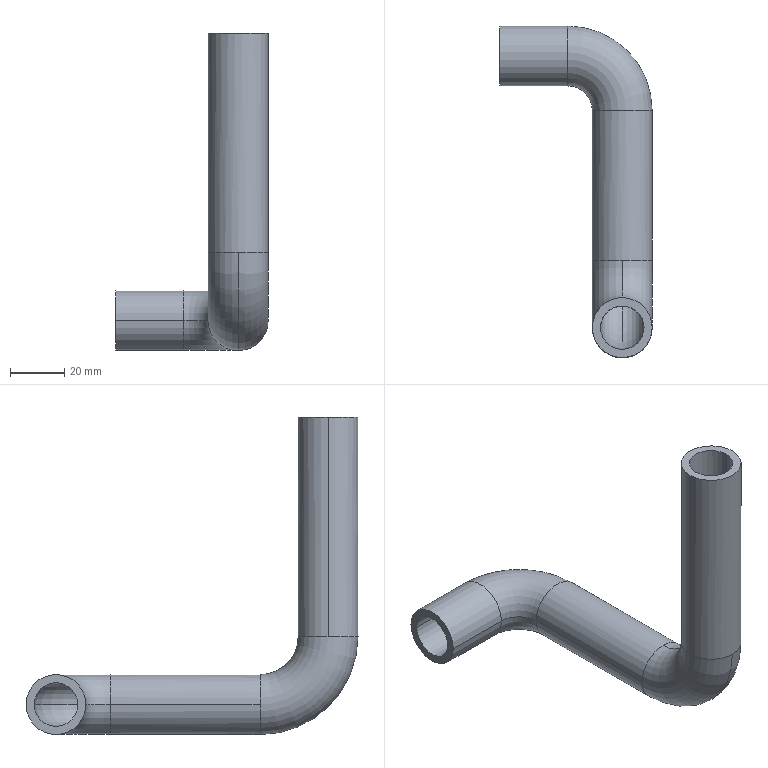Part | SolidWorks | features Sweep 2 | 1 solid | 22 faces | box 56 x 122 x 116.5 mm | volume 41399 mm3 | cylinder 12 | torus 8 | plane 2 | commonest cylinder face diameters 16 x6 22 x6
STEP:
#1=CARTESIAN_POINT('',(53.,-75.,0.));
#2=VERTEX_POINT('',#1);
#3=CARTESIAN_POINT('',(45.,-75.,-8.));
#4=VERTEX_POINT('',#3);
#5=CARTESIAN_POINT('',(45.,-75.,0.));
#6=DIRECTION('',(0.,1.,0.));
#7=DIRECTION('',(1.,0.,0.));
#8=AXIS2_PLACEMENT_3D('',#5,#6,#7);
#9=CIRCLE('',#8,8.);
#10=EDGE_CURVE('',#2,#4,#9,.T.);
#11=ORIENTED_EDGE('',*,*,#10,.T.);
#12=CARTESIAN_POINT('',(45.,-108.,25.));
#13=VERTEX_POINT('',#12);
#14=CARTESIAN_POINT('',(45.,-75.,25.));
#15=DIRECTION('',(-1.,0.,0.));
#16=DIRECTION('',(0.,0.,1.));
#17=AXIS2_PLACEMENT_3D('',#14,#15,#16);
#18=CIRCLE('',#17,33.);
#19=EDGE_CURVE('',#4,#13,#18,.T.);
#20=ORIENTED_EDGE('',*,*,#19,.T.);
#21=CARTESIAN_POINT('',(53.,-100.,25.));
#22=VERTEX_POINT('',#21);
#23=CARTESIAN_POINT('',(45.,-100.,25.));
#24=DIRECTION('',(0.,0.,-1.));
#25=DIRECTION('',(1.,0.,0.));
#26=AXIS2_PLACEMENT_3D('',#23,#24,#25);
#27=CIRCLE('',#26,8.);
#28=EDGE_CURVE('',#22,#13,#27,.T.);
#29=ORIENTED_EDGE('',*,*,#28,.F.);
#30=CARTESIAN_POINT('',(45.,-92.,25.));
#31=VERTEX_POINT('',#30);
#32=CARTESIAN_POINT('',(45.,-100.,25.));
#33=DIRECTION('',(0.,0.,-1.));
#34=DIRECTION('',(1.,0.,0.));
#35=AXIS2_PLACEMENT_3D('',#32,#33,#34);
#36=CIRCLE('',#35,8.);
#37=EDGE_CURVE('',#31,#22,#36,.T.);
#38=ORIENTED_EDGE('',*,*,#37,.F.);
#39=CARTESIAN_POINT('',(45.,-75.,8.));
#40=VERTEX_POINT('',#39);
#41=CARTESIAN_POINT('',(45.,-75.,25.));
#42=DIRECTION('',(-1.,0.,0.));
#43=DIRECTION('',(0.,0.,1.));
#44=AXIS2_PLACEMENT_3D('',#41,#42,#43);
#45=CIRCLE('',#44,17.);
#46=EDGE_CURVE('',#40,#31,#45,.T.);
#47=ORIENTED_EDGE('',*,*,#46,.F.);
#48=CARTESIAN_POINT('',(45.,-75.,0.));
#49=DIRECTION('',(0.,1.,0.));
#50=DIRECTION('',(1.,0.,0.));
#51=AXIS2_PLACEMENT_3D('',#48,#49,#50);
#52=CIRCLE('',#51,8.);
#53=EDGE_CURVE('',#40,#2,#52,.T.);
#54=ORIENTED_EDGE('',*,*,#53,.T.);
#55=EDGE_LOOP('',(#11,#20,#29,#38,#47,#54));
#56=FACE_OUTER_BOUND('',#55,.T.);
#57=CARTESIAN_POINT('',(45.,-75.,25.));
#58=DIRECTION('',(-1.,0.,0.));
#59=DIRECTION('',(0.,0.,1.));
#60=AXIS2_PLACEMENT_3D('',#57,#58,#59);
#61=TOROIDAL_SURFACE('',#60,25.,8.);
#62=ADVANCED_FACE('',(#56),#61,.F.);
#63=CARTESIAN_POINT('',(34.,-75.,0.));
#64=VERTEX_POINT('',#63);
#65=CARTESIAN_POINT('',(45.,-75.,-11.));
#66=VERTEX_POINT('',#65);
#67=CARTESIAN_POINT('',(45.,-75.,0.));
#68=DIRECTION('',(0.,-1.,0.));
#69=DIRECTION('',(1.,0.,0.));
#70=AXIS2_PLACEMENT_3D('',#67,#68,#69);
#71=CIRCLE('',#70,11.);
#72=EDGE_CURVE('',#64,#66,#71,.T.);
#73=ORIENTED_EDGE('',*,*,#72,.T.);
#74=CARTESIAN_POINT('',(45.,-111.,25.));
#75=VERTEX_POINT('',#74);
#76=CARTESIAN_POINT('',(45.,-75.,25.));
#77=DIRECTION('',(-1.,0.,0.));
#78=DIRECTION('',(0.,0.,1.));
#79=AXIS2_PLACEMENT_3D('',#76,#77,#78);
#80=CIRCLE('',#79,36.);
#81=EDGE_CURVE('',#66,#75,#80,.T.);
#82=ORIENTED_EDGE('',*,*,#81,.T.);
#83=CARTESIAN_POINT('',(34.,-100.,25.));
#84=VERTEX_POINT('',#83);
#85=CARTESIAN_POINT('',(45.,-100.,25.));
#86=DIRECTION('',(0.,0.,1.));
#87=DIRECTION('',(1.,0.,0.));
#88=AXIS2_PLACEMENT_3D('',#85,#86,#87);
#89=CIRCLE('',#88,11.);
#90=EDGE_CURVE('',#84,#75,#89,.T.);
#91=ORIENTED_EDGE('',*,*,#90,.F.);
#92=CARTESIAN_POINT('',(45.,-89.,25.));
#93=VERTEX_POINT('',#92);
#94=CARTESIAN_POINT('',(45.,-100.,25.));
#95=DIRECTION('',(0.,0.,1.));
#96=DIRECTION('',(1.,0.,0.));
#97=AXIS2_PLACEMENT_3D('',#94,#95,#96);
#98=CIRCLE('',#97,11.);
#99=EDGE_CURVE('',#93,#84,#98,.T.);
#100=ORIENTED_EDGE('',*,*,#99,.F.);
#101=CARTESIAN_POINT('',(45.,-75.,11.));
#102=VERTEX_POINT('',#101);
#103=CARTESIAN_POINT('',(45.,-75.,25.));
#104=DIRECTION('',(-1.,0.,0.));
#105=DIRECTION('',(0.,0.,1.));
#106=AXIS2_PLACEMENT_3D('',#103,#104,#105);
#107=CIRCLE('',#106,14.);
#108=EDGE_CURVE('',#102,#93,#107,.T.);
#109=ORIENTED_EDGE('',*,*,#108,.F.);
#110=CARTESIAN_POINT('',(45.,-75.,0.));
#111=DIRECTION('',(0.,-1.,0.));
#112=DIRECTION('',(1.,0.,0.));
#113=AXIS2_PLACEMENT_3D('',#110,#111,#112);
#114=CIRCLE('',#113,11.);
#115=EDGE_CURVE('',#102,#64,#114,.T.);
#116=ORIENTED_EDGE('',*,*,#115,.T.);
#117=EDGE_LOOP('',(#73,#82,#91,#100,#109,#116));
#118=FACE_OUTER_BOUND('',#117,.T.);
#119=CARTESIAN_POINT('',(45.,-75.,25.));
#120=DIRECTION('',(-1.,0.,0.));
#121=DIRECTION('',(0.,0.,1.));
#122=AXIS2_PLACEMENT_3D('',#119,#120,#121);
#123=TOROIDAL_SURFACE('',#122,25.,11.);
#124=ADVANCED_FACE('',(#118),#123,.T.);
#125=CARTESIAN_POINT('',(25.,-8.,0.));
#126=VERTEX_POINT('',#125);
#127=CARTESIAN_POINT('',(25.,8.,0.));
#128=VERTEX_POINT('',#127);
#129=CARTESIAN_POINT('',(25.,0.,0.));
#130=DIRECTION('',(-1.,0.,0.));
#131=DIRECTION('',(0.,0.,-1.));
#132=AXIS2_PLACEMENT_3D('',#129,#130,#131);
#133=CIRCLE('',#132,8.);
#134=EDGE_CURVE('',#126,#128,#133,.T.);
#135=ORIENTED_EDGE('',*,*,#134,.T.);
#136=CARTESIAN_POINT('',(53.,-20.,0.));
#137=VERTEX_POINT('',#136);
#138=CARTESIAN_POINT('',(25.,-20.,0.));
#139=DIRECTION('',(0.,0.,-1.));
#140=DIRECTION('',(-1.,0.,0.));
#141=AXIS2_PLACEMENT_3D('',#138,#139,#140);
#142=CIRCLE('',#141,28.);
#143=EDGE_CURVE('',#128,#137,#142,.T.);
#144=ORIENTED_EDGE('',*,*,#143,.T.);
#145=CARTESIAN_POINT('',(37.,-20.,0.));
#146=VERTEX_POINT('',#145);
#147=CARTESIAN_POINT('',(45.,-20.,0.));
#148=DIRECTION('',(0.,1.,0.));
#149=DIRECTION('',(0.,0.,-1.));
#150=AXIS2_PLACEMENT_3D('',#147,#148,#149);
#151=CIRCLE('',#150,8.);
#152=EDGE_CURVE('',#146,#137,#151,.T.);
#153=ORIENTED_EDGE('',*,*,#152,.F.);
#154=CARTESIAN_POINT('',(25.,-20.,0.));
#155=DIRECTION('',(0.,0.,-1.));
#156=DIRECTION('',(-1.,0.,0.));
#157=AXIS2_PLACEMENT_3D('',#154,#155,#156);
#158=CIRCLE('',#157,12.);
#159=EDGE_CURVE('',#126,#146,#158,.T.);
#160=ORIENTED_EDGE('',*,*,#159,.F.);
#161=EDGE_LOOP('',(#135,#144,#153,#160));
#162=FACE_OUTER_BOUND('',#161,.T.);
#163=CARTESIAN_POINT('',(25.,-20.,0.));
#164=DIRECTION('',(0.,0.,-1.));
#165=DIRECTION('',(-1.,0.,0.));
#166=AXIS2_PLACEMENT_3D('',#163,#164,#165);
#167=TOROIDAL_SURFACE('',#166,20.,8.);
#168=ADVANCED_FACE('',(#162),#167,.F.);
#169=CARTESIAN_POINT('',(25.,-11.,0.));
#170=VERTEX_POINT('',#169);
#171=CARTESIAN_POINT('',(25.,11.,0.));
#172=VERTEX_POINT('',#171);
#173=CARTESIAN_POINT('',(25.,0.,0.));
#174=DIRECTION('',(1.,0.,0.));
#175=DIRECTION('',(0.,0.,-1.));
#176=AXIS2_PLACEMENT_3D('',#173,#174,#175);
#177=CIRCLE('',#176,11.);
#178=EDGE_CURVE('',#170,#172,#177,.T.);
#179=ORIENTED_EDGE('',*,*,#178,.T.);
#180=CARTESIAN_POINT('',(56.,-20.,0.));
#181=VERTEX_POINT('',#180);
#182=CARTESIAN_POINT('',(25.,-20.,0.));
#183=DIRECTION('',(0.,0.,-1.));
#184=DIRECTION('',(-1.,0.,0.));
#185=AXIS2_PLACEMENT_3D('',#182,#183,#184);
#186=CIRCLE('',#185,31.);
#187=EDGE_CURVE('',#172,#181,#186,.T.);
#188=ORIENTED_EDGE('',*,*,#187,.T.);
#189=CARTESIAN_POINT('',(34.,-20.,0.));
#190=VERTEX_POINT('',#189);
#191=CARTESIAN_POINT('',(45.,-20.,0.));
#192=DIRECTION('',(0.,-1.,0.));
#193=DIRECTION('',(0.,0.,-1.));
#194=AXIS2_PLACEMENT_3D('',#191,#192,#193);
#195=CIRCLE('',#194,11.);
#196=EDGE_CURVE('',#190,#181,#195,.T.);
#197=ORIENTED_EDGE('',*,*,#196,.F.);
#198=CARTESIAN_POINT('',(25.,-20.,0.));
#199=DIRECTION('',(0.,0.,-1.));
#200=DIRECTION('',(-1.,0.,0.));
#201=AXIS2_PLACEMENT_3D('',#198,#199,#200);
#202=CIRCLE('',#201,9.);
#203=EDGE_CURVE('',#170,#190,#202,.T.);
#204=ORIENTED_EDGE('',*,*,#203,.F.);
#205=EDGE_LOOP('',(#179,#188,#197,#204));
#206=FACE_OUTER_BOUND('',#205,.T.);
#207=CARTESIAN_POINT('',(25.,-20.,0.));
#208=DIRECTION('',(0.,0.,-1.));
#209=DIRECTION('',(-1.,0.,0.));
#210=AXIS2_PLACEMENT_3D('',#207,#208,#209);
#211=TOROIDAL_SURFACE('',#210,20.,11.);
#212=ADVANCED_FACE('',(#206),#211,.T.);
#213=ORIENTED_EDGE('',*,*,#28,.T.);
#214=CARTESIAN_POINT('',(37.,-100.,25.));
#215=VERTEX_POINT('',#214);
#216=CARTESIAN_POINT('',(45.,-100.,25.));
#217=DIRECTION('',(0.,0.,-1.));
#218=DIRECTION('',(1.,0.,0.));
#219=AXIS2_PLACEMENT_3D('',#216,#217,#218);
#220=CIRCLE('',#219,8.);
#221=EDGE_CURVE('',#13,#215,#220,.T.);
#222=ORIENTED_EDGE('',*,*,#221,.T.);
#223=CARTESIAN_POINT('',(37.,-100.,105.5));
#224=VERTEX_POINT('',#223);
#225=CARTESIAN_POINT('',(37.,-100.,25.));
#226=DIRECTION('',(0.,0.,1.));
#227=VECTOR('',#226,1000.);
#228=LINE('',#225,#227);
#229=EDGE_CURVE('',#215,#224,#228,.T.);
#230=ORIENTED_EDGE('',*,*,#229,.T.);
#231=CARTESIAN_POINT('',(53.,-100.,105.5));
#232=VERTEX_POINT('',#231);
#233=CARTESIAN_POINT('',(45.,-100.,105.5));
#234=DIRECTION('',(0.,0.,-1.));
#235=DIRECTION('',(1.,0.,0.));
#236=AXIS2_PLACEMENT_3D('',#233,#234,#235);
#237=CIRCLE('',#236,8.);
#238=EDGE_CURVE('',#232,#224,#237,.T.);
#239=ORIENTED_EDGE('',*,*,#238,.F.);
#240=CARTESIAN_POINT('',(53.,-100.,25.));
#241=DIRECTION('',(0.,0.,1.));
#242=VECTOR('',#241,1000.);
#243=LINE('',#240,#242);
#244=EDGE_CURVE('',#22,#232,#243,.T.);
#245=ORIENTED_EDGE('',*,*,#244,.F.);
#246=EDGE_LOOP('',(#213,#222,#230,#239,#245));
#247=FACE_OUTER_BOUND('',#246,.T.);
#248=CARTESIAN_POINT('',(45.,-100.,25.));
#249=DIRECTION('',(0.,0.,1.));
#250=DIRECTION('',(1.,0.,0.));
#251=AXIS2_PLACEMENT_3D('',#248,#249,#250);
#252=CYLINDRICAL_SURFACE('',#251,8.);
#253=ADVANCED_FACE('',(#247),#252,.F.);
#254=CARTESIAN_POINT('',(56.,-100.,25.));
#255=VERTEX_POINT('',#254);
#256=CARTESIAN_POINT('',(45.,-100.,25.));
#257=DIRECTION('',(0.,0.,1.));
#258=DIRECTION('',(1.,0.,0.));
#259=AXIS2_PLACEMENT_3D('',#256,#257,#258);
#260=CIRCLE('',#259,11.);
#261=EDGE_CURVE('',#255,#93,#260,.T.);
#262=ORIENTED_EDGE('',*,*,#261,.T.);
#263=ORIENTED_EDGE('',*,*,#99,.T.);
#264=CARTESIAN_POINT('',(34.,-100.,105.5));
#265=VERTEX_POINT('',#264);
#266=CARTESIAN_POINT('',(34.,-100.,25.));
#267=DIRECTION('',(0.,0.,1.));
#268=VECTOR('',#267,1000.);
#269=LINE('',#266,#268);
#270=EDGE_CURVE('',#84,#265,#269,.T.);
#271=ORIENTED_EDGE('',*,*,#270,.T.);
#272=CARTESIAN_POINT('',(56.,-100.,105.5));
#273=VERTEX_POINT('',#272);
#274=CARTESIAN_POINT('',(45.,-100.,105.5));
#275=DIRECTION('',(0.,0.,1.));
#276=DIRECTION('',(1.,0.,0.));
#277=AXIS2_PLACEMENT_3D('',#274,#275,#276);
#278=CIRCLE('',#277,11.);
#279=EDGE_CURVE('',#273,#265,#278,.T.);
#280=ORIENTED_EDGE('',*,*,#279,.F.);
#281=CARTESIAN_POINT('',(56.,-100.,25.));
#282=DIRECTION('',(0.,0.,1.));
#283=VECTOR('',#282,1000.);
#284=LINE('',#281,#283);
#285=EDGE_CURVE('',#255,#273,#284,.T.);
#286=ORIENTED_EDGE('',*,*,#285,.F.);
#287=EDGE_LOOP('',(#262,#263,#271,#280,#286));
#288=FACE_OUTER_BOUND('',#287,.T.);
#289=CARTESIAN_POINT('',(45.,-100.,25.));
#290=DIRECTION('',(0.,0.,1.));
#291=DIRECTION('',(1.,0.,0.));
#292=AXIS2_PLACEMENT_3D('',#289,#290,#291);
#293=CYLINDRICAL_SURFACE('',#292,11.);
#294=ADVANCED_FACE('',(#288),#293,.T.);
#295=CARTESIAN_POINT('',(45.,-20.,0.));
#296=DIRECTION('',(0.,1.,0.));
#297=DIRECTION('',(0.,0.,-1.));
#298=AXIS2_PLACEMENT_3D('',#295,#296,#297);
#299=CIRCLE('',#298,8.);
#300=EDGE_CURVE('',#137,#146,#299,.T.);
#301=ORIENTED_EDGE('',*,*,#300,.T.);
#302=CARTESIAN_POINT('',(37.,-75.,0.));
#303=VERTEX_POINT('',#302);
#304=CARTESIAN_POINT('',(37.,-20.,0.));
#305=DIRECTION('',(0.,-1.,0.));
#306=VECTOR('',#305,1000.);
#307=LINE('',#304,#306);
#308=EDGE_CURVE('',#146,#303,#307,.T.);
#309=ORIENTED_EDGE('',*,*,#308,.T.);
#310=CARTESIAN_POINT('',(45.,-75.,0.));
#311=DIRECTION('',(0.,1.,0.));
#312=DIRECTION('',(1.,0.,0.));
#313=AXIS2_PLACEMENT_3D('',#310,#311,#312);
#314=CIRCLE('',#313,8.);
#315=EDGE_CURVE('',#4,#303,#314,.T.);
#316=ORIENTED_EDGE('',*,*,#315,.F.);
#317=ORIENTED_EDGE('',*,*,#10,.F.);
#318=CARTESIAN_POINT('',(53.,-20.,0.));
#319=DIRECTION('',(0.,-1.,0.));
#320=VECTOR('',#319,1000.);
#321=LINE('',#318,#320);
#322=EDGE_CURVE('',#137,#2,#321,.T.);
#323=ORIENTED_EDGE('',*,*,#322,.F.);
#324=EDGE_LOOP('',(#301,#309,#316,#317,#323));
#325=FACE_OUTER_BOUND('',#324,.T.);
#326=CARTESIAN_POINT('',(45.,-20.,0.));
#327=DIRECTION('',(0.,-1.,0.));
#328=DIRECTION('',(1.,0.,0.));
#329=AXIS2_PLACEMENT_3D('',#326,#327,#328);
#330=CYLINDRICAL_SURFACE('',#329,8.);
#331=ADVANCED_FACE('',(#325),#330,.F.);
#332=CARTESIAN_POINT('',(0.,8.,0.));
#333=VERTEX_POINT('',#332);
#334=CARTESIAN_POINT('',(0.,-8.,0.));
#335=VERTEX_POINT('',#334);
#336=CARTESIAN_POINT('',(0.,0.,0.));
#337=DIRECTION('',(-1.,0.,0.));
#338=DIRECTION('',(0.,0.,-1.));
#339=AXIS2_PLACEMENT_3D('',#336,#337,#338);
#340=CIRCLE('',#339,8.);
#341=EDGE_CURVE('',#333,#335,#340,.T.);
#342=ORIENTED_EDGE('',*,*,#341,.T.);
#343=CARTESIAN_POINT('',(0.,-8.,0.));
#344=DIRECTION('',(1.,0.,0.));
#345=VECTOR('',#344,1000.);
#346=LINE('',#343,#345);
#347=EDGE_CURVE('',#335,#126,#346,.T.);
#348=ORIENTED_EDGE('',*,*,#347,.T.);
#349=CARTESIAN_POINT('',(25.,0.,0.));
#350=DIRECTION('',(-1.,0.,0.));
#351=DIRECTION('',(0.,0.,-1.));
#352=AXIS2_PLACEMENT_3D('',#349,#350,#351);
#353=CIRCLE('',#352,8.);
#354=EDGE_CURVE('',#128,#126,#353,.T.);
#355=ORIENTED_EDGE('',*,*,#354,.F.);
#356=CARTESIAN_POINT('',(0.,8.,0.));
#357=DIRECTION('',(1.,0.,0.));
#358=VECTOR('',#357,1000.);
#359=LINE('',#356,#358);
#360=EDGE_CURVE('',#333,#128,#359,.T.);
#361=ORIENTED_EDGE('',*,*,#360,.F.);
#362=EDGE_LOOP('',(#342,#348,#355,#361));
#363=FACE_OUTER_BOUND('',#362,.T.);
#364=CARTESIAN_POINT('',(0.,0.,0.));
#365=DIRECTION('',(1.,0.,0.));
#366=DIRECTION('',(0.,1.,0.));
#367=AXIS2_PLACEMENT_3D('',#364,#365,#366);
#368=CYLINDRICAL_SURFACE('',#367,8.);
#369=ADVANCED_FACE('',(#363),#368,.F.);
#370=CARTESIAN_POINT('',(45.,-20.,0.));
#371=DIRECTION('',(0.,-1.,0.));
#372=DIRECTION('',(0.,0.,-1.));
#373=AXIS2_PLACEMENT_3D('',#370,#371,#372);
#374=CIRCLE('',#373,11.);
#375=EDGE_CURVE('',#181,#190,#374,.T.);
#376=ORIENTED_EDGE('',*,*,#375,.T.);
#377=CARTESIAN_POINT('',(34.,-20.,0.));
#378=DIRECTION('',(0.,-1.,0.));
#379=VECTOR('',#378,1000.);
#380=LINE('',#377,#379);
#381=EDGE_CURVE('',#190,#64,#380,.T.);
#382=ORIENTED_EDGE('',*,*,#381,.T.);
#383=ORIENTED_EDGE('',*,*,#115,.F.);
#384=CARTESIAN_POINT('',(56.,-75.,0.));
#385=VERTEX_POINT('',#384);
#386=CARTESIAN_POINT('',(45.,-75.,0.));
#387=DIRECTION('',(0.,-1.,0.));
#388=DIRECTION('',(1.,0.,0.));
#389=AXIS2_PLACEMENT_3D('',#386,#387,#388);
#390=CIRCLE('',#389,11.);
#391=EDGE_CURVE('',#385,#102,#390,.T.);
#392=ORIENTED_EDGE('',*,*,#391,.F.);
#393=CARTESIAN_POINT('',(56.,-20.,0.));
#394=DIRECTION('',(0.,-1.,0.));
#395=VECTOR('',#394,1000.);
#396=LINE('',#393,#395);
#397=EDGE_CURVE('',#181,#385,#396,.T.);
#398=ORIENTED_EDGE('',*,*,#397,.F.);
#399=EDGE_LOOP('',(#376,#382,#383,#392,#398));
#400=FACE_OUTER_BOUND('',#399,.T.);
#401=CARTESIAN_POINT('',(45.,-20.,0.));
#402=DIRECTION('',(0.,-1.,0.));
#403=DIRECTION('',(1.,0.,0.));
#404=AXIS2_PLACEMENT_3D('',#401,#402,#403);
#405=CYLINDRICAL_SURFACE('',#404,11.);
#406=ADVANCED_FACE('',(#400),#405,.T.);
#407=CARTESIAN_POINT('',(0.,11.,0.));
#408=VERTEX_POINT('',#407);
#409=CARTESIAN_POINT('',(0.,-11.,0.));
#410=VERTEX_POINT('',#409);
#411=CARTESIAN_POINT('',(0.,0.,0.));
#412=DIRECTION('',(1.,0.,0.));
#413=DIRECTION('',(0.,0.,-1.));
#414=AXIS2_PLACEMENT_3D('',#411,#412,#413);
#415=CIRCLE('',#414,11.);
#416=EDGE_CURVE('',#408,#410,#415,.T.);
#417=ORIENTED_EDGE('',*,*,#416,.T.);
#418=CARTESIAN_POINT('',(0.,-11.,0.));
#419=DIRECTION('',(1.,0.,0.));
#420=VECTOR('',#419,1000.);
#421=LINE('',#418,#420);
#422=EDGE_CURVE('',#410,#170,#421,.T.);
#423=ORIENTED_EDGE('',*,*,#422,.T.);
#424=CARTESIAN_POINT('',(25.,0.,0.));
#425=DIRECTION('',(1.,0.,0.));
#426=DIRECTION('',(0.,0.,-1.));
#427=AXIS2_PLACEMENT_3D('',#424,#425,#426);
#428=CIRCLE('',#427,11.);
#429=EDGE_CURVE('',#172,#170,#428,.T.);
#430=ORIENTED_EDGE('',*,*,#429,.F.);
#431=CARTESIAN_POINT('',(0.,11.,0.));
#432=DIRECTION('',(1.,0.,0.));
#433=VECTOR('',#432,1000.);
#434=LINE('',#431,#433);
#435=EDGE_CURVE('',#408,#172,#434,.T.);
#436=ORIENTED_EDGE('',*,*,#435,.F.);
#437=EDGE_LOOP('',(#417,#423,#430,#436));
#438=FACE_OUTER_BOUND('',#437,.T.);
#439=CARTESIAN_POINT('',(0.,0.,0.));
#440=DIRECTION('',(1.,0.,0.));
#441=DIRECTION('',(0.,1.,0.));
#442=AXIS2_PLACEMENT_3D('',#439,#440,#441);
#443=CYLINDRICAL_SURFACE('',#442,11.);
#444=ADVANCED_FACE('',(#438),#443,.T.);
#445=ORIENTED_EDGE('',*,*,#308,.F.);
#446=ORIENTED_EDGE('',*,*,#152,.T.);
#447=ORIENTED_EDGE('',*,*,#322,.T.);
#448=ORIENTED_EDGE('',*,*,#53,.F.);
#449=CARTESIAN_POINT('',(45.,-75.,0.));
#450=DIRECTION('',(0.,1.,0.));
#451=DIRECTION('',(1.,0.,0.));
#452=AXIS2_PLACEMENT_3D('',#449,#450,#451);
#453=CIRCLE('',#452,8.);
#454=EDGE_CURVE('',#303,#40,#453,.T.);
#455=ORIENTED_EDGE('',*,*,#454,.F.);
#456=EDGE_LOOP('',(#445,#446,#447,#448,#455));
#457=FACE_OUTER_BOUND('',#456,.T.);
#458=CARTESIAN_POINT('',(45.,-20.,0.));
#459=DIRECTION('',(0.,-1.,0.));
#460=DIRECTION('',(1.,0.,0.));
#461=AXIS2_PLACEMENT_3D('',#458,#459,#460);
#462=CYLINDRICAL_SURFACE('',#461,8.);
#463=ADVANCED_FACE('',(#457),#462,.F.);
#464=ORIENTED_EDGE('',*,*,#143,.F.);
#465=ORIENTED_EDGE('',*,*,#354,.T.);
#466=ORIENTED_EDGE('',*,*,#159,.T.);
#467=ORIENTED_EDGE('',*,*,#300,.F.);
#468=EDGE_LOOP('',(#464,#465,#466,#467));
#469=FACE_OUTER_BOUND('',#468,.T.);
#470=CARTESIAN_POINT('',(25.,-20.,0.));
#471=DIRECTION('',(0.,0.,-1.));
#472=DIRECTION('',(-1.,0.,0.));
#473=AXIS2_PLACEMENT_3D('',#470,#471,#472);
#474=TOROIDAL_SURFACE('',#473,20.,8.);
#475=ADVANCED_FACE('',(#469),#474,.F.);
#476=ORIENTED_EDGE('',*,*,#347,.F.);
#477=CARTESIAN_POINT('',(0.,0.,0.));
#478=DIRECTION('',(-1.,0.,0.));
#479=DIRECTION('',(0.,0.,-1.));
#480=AXIS2_PLACEMENT_3D('',#477,#478,#479);
#481=CIRCLE('',#480,8.);
#482=EDGE_CURVE('',#335,#333,#481,.T.);
#483=ORIENTED_EDGE('',*,*,#482,.T.);
#484=ORIENTED_EDGE('',*,*,#360,.T.);
#485=ORIENTED_EDGE('',*,*,#134,.F.);
#486=EDGE_LOOP('',(#476,#483,#484,#485));
#487=FACE_OUTER_BOUND('',#486,.T.);
#488=CARTESIAN_POINT('',(0.,0.,0.));
#489=DIRECTION('',(1.,0.,0.));
#490=DIRECTION('',(0.,1.,0.));
#491=AXIS2_PLACEMENT_3D('',#488,#489,#490);
#492=CYLINDRICAL_SURFACE('',#491,8.);
#493=ADVANCED_FACE('',(#487),#492,.F.);
#494=ORIENTED_EDGE('',*,*,#341,.F.);
#495=ORIENTED_EDGE('',*,*,#482,.F.);
#496=EDGE_LOOP('',(#494,#495));
#497=FACE_BOUND('',#496,.T.);
#498=ORIENTED_EDGE('',*,*,#416,.F.);
#499=CARTESIAN_POINT('',(0.,0.,0.));
#500=DIRECTION('',(1.,0.,0.));
#501=DIRECTION('',(0.,0.,-1.));
#502=AXIS2_PLACEMENT_3D('',#499,#500,#501);
#503=CIRCLE('',#502,11.);
#504=EDGE_CURVE('',#410,#408,#503,.T.);
#505=ORIENTED_EDGE('',*,*,#504,.F.);
#506=EDGE_LOOP('',(#498,#505));
#507=FACE_OUTER_BOUND('',#506,.T.);
#508=CARTESIAN_POINT('',(0.,0.,0.));
#509=DIRECTION('',(1.,0.,0.));
#510=DIRECTION('',(0.,0.,-1.));
#511=AXIS2_PLACEMENT_3D('',#508,#509,#510);
#512=PLANE('',#511);
#513=ADVANCED_FACE('',(#497,#507),#512,.F.);
#514=ORIENTED_EDGE('',*,*,#381,.F.);
#515=ORIENTED_EDGE('',*,*,#196,.T.);
#516=ORIENTED_EDGE('',*,*,#397,.T.);
#517=CARTESIAN_POINT('',(45.,-75.,0.));
#518=DIRECTION('',(0.,-1.,0.));
#519=DIRECTION('',(1.,0.,0.));
#520=AXIS2_PLACEMENT_3D('',#517,#518,#519);
#521=CIRCLE('',#520,11.);
#522=EDGE_CURVE('',#66,#385,#521,.T.);
#523=ORIENTED_EDGE('',*,*,#522,.F.);
#524=ORIENTED_EDGE('',*,*,#72,.F.);
#525=EDGE_LOOP('',(#514,#515,#516,#523,#524));
#526=FACE_OUTER_BOUND('',#525,.T.);
#527=CARTESIAN_POINT('',(45.,-20.,0.));
#528=DIRECTION('',(0.,-1.,0.));
#529=DIRECTION('',(1.,0.,0.));
#530=AXIS2_PLACEMENT_3D('',#527,#528,#529);
#531=CYLINDRICAL_SURFACE('',#530,11.);
#532=ADVANCED_FACE('',(#526),#531,.T.);
#533=ORIENTED_EDGE('',*,*,#187,.F.);
#534=ORIENTED_EDGE('',*,*,#429,.T.);
#535=ORIENTED_EDGE('',*,*,#203,.T.);
#536=ORIENTED_EDGE('',*,*,#375,.F.);
#537=EDGE_LOOP('',(#533,#534,#535,#536));
#538=FACE_OUTER_BOUND('',#537,.T.);
#539=CARTESIAN_POINT('',(25.,-20.,0.));
#540=DIRECTION('',(0.,0.,-1.));
#541=DIRECTION('',(-1.,0.,0.));
#542=AXIS2_PLACEMENT_3D('',#539,#540,#541);
#543=TOROIDAL_SURFACE('',#542,20.,11.);
#544=ADVANCED_FACE('',(#538),#543,.T.);
#545=ORIENTED_EDGE('',*,*,#422,.F.);
#546=ORIENTED_EDGE('',*,*,#504,.T.);
#547=ORIENTED_EDGE('',*,*,#435,.T.);
#548=ORIENTED_EDGE('',*,*,#178,.F.);
#549=EDGE_LOOP('',(#545,#546,#547,#548));
#550=FACE_OUTER_BOUND('',#549,.T.);
#551=CARTESIAN_POINT('',(0.,0.,0.));
#552=DIRECTION('',(1.,0.,0.));
#553=DIRECTION('',(0.,1.,0.));
#554=AXIS2_PLACEMENT_3D('',#551,#552,#553);
#555=CYLINDRICAL_SURFACE('',#554,11.);
#556=ADVANCED_FACE('',(#550),#555,.T.);
#557=ORIENTED_EDGE('',*,*,#229,.F.);
#558=CARTESIAN_POINT('',(45.,-100.,25.));
#559=DIRECTION('',(0.,0.,-1.));
#560=DIRECTION('',(1.,0.,0.));
#561=AXIS2_PLACEMENT_3D('',#558,#559,#560);
#562=CIRCLE('',#561,8.);
#563=EDGE_CURVE('',#215,#31,#562,.T.);
#564=ORIENTED_EDGE('',*,*,#563,.T.);
#565=ORIENTED_EDGE('',*,*,#37,.T.);
#566=ORIENTED_EDGE('',*,*,#244,.T.);
#567=CARTESIAN_POINT('',(45.,-100.,105.5));
#568=DIRECTION('',(0.,0.,-1.));
#569=DIRECTION('',(1.,0.,0.));
#570=AXIS2_PLACEMENT_3D('',#567,#568,#569);
#571=CIRCLE('',#570,8.);
#572=EDGE_CURVE('',#224,#232,#571,.T.);
#573=ORIENTED_EDGE('',*,*,#572,.F.);
#574=EDGE_LOOP('',(#557,#564,#565,#566,#573));
#575=FACE_OUTER_BOUND('',#574,.T.);
#576=CARTESIAN_POINT('',(45.,-100.,25.));
#577=DIRECTION('',(0.,0.,1.));
#578=DIRECTION('',(1.,0.,0.));
#579=AXIS2_PLACEMENT_3D('',#576,#577,#578);
#580=CYLINDRICAL_SURFACE('',#579,8.);
#581=ADVANCED_FACE('',(#575),#580,.F.);
#582=ORIENTED_EDGE('',*,*,#19,.F.);
#583=ORIENTED_EDGE('',*,*,#315,.T.);
#584=ORIENTED_EDGE('',*,*,#454,.T.);
#585=ORIENTED_EDGE('',*,*,#46,.T.);
#586=ORIENTED_EDGE('',*,*,#563,.F.);
#587=ORIENTED_EDGE('',*,*,#221,.F.);
#588=EDGE_LOOP('',(#582,#583,#584,#585,#586,#587));
#589=FACE_OUTER_BOUND('',#588,.T.);
#590=CARTESIAN_POINT('',(45.,-75.,25.));
#591=DIRECTION('',(-1.,0.,0.));
#592=DIRECTION('',(0.,0.,1.));
#593=AXIS2_PLACEMENT_3D('',#590,#591,#592);
#594=TOROIDAL_SURFACE('',#593,25.,8.);
#595=ADVANCED_FACE('',(#589),#594,.F.);
#596=ORIENTED_EDGE('',*,*,#238,.T.);
#597=ORIENTED_EDGE('',*,*,#572,.T.);
#598=EDGE_LOOP('',(#596,#597));
#599=FACE_BOUND('',#598,.T.);
#600=ORIENTED_EDGE('',*,*,#279,.T.);
#601=CARTESIAN_POINT('',(45.,-100.,105.5));
#602=DIRECTION('',(0.,0.,1.));
#603=DIRECTION('',(1.,0.,0.));
#604=AXIS2_PLACEMENT_3D('',#601,#602,#603);
#605=CIRCLE('',#604,11.);
#606=EDGE_CURVE('',#265,#273,#605,.T.);
#607=ORIENTED_EDGE('',*,*,#606,.T.);
#608=EDGE_LOOP('',(#600,#607));
#609=FACE_OUTER_BOUND('',#608,.T.);
#610=CARTESIAN_POINT('',(45.,-100.,105.5));
#611=DIRECTION('',(0.,0.,1.));
#612=DIRECTION('',(1.,0.,0.));
#613=AXIS2_PLACEMENT_3D('',#610,#611,#612);
#614=PLANE('',#613);
#615=ADVANCED_FACE('',(#599,#609),#614,.T.);
#616=ORIENTED_EDGE('',*,*,#270,.F.);
#617=ORIENTED_EDGE('',*,*,#90,.T.);
#618=CARTESIAN_POINT('',(45.,-100.,25.));
#619=DIRECTION('',(0.,0.,1.));
#620=DIRECTION('',(1.,0.,0.));
#621=AXIS2_PLACEMENT_3D('',#618,#619,#620);
#622=CIRCLE('',#621,11.);
#623=EDGE_CURVE('',#75,#255,#622,.T.);
#624=ORIENTED_EDGE('',*,*,#623,.T.);
#625=ORIENTED_EDGE('',*,*,#285,.T.);
#626=ORIENTED_EDGE('',*,*,#606,.F.);
#627=EDGE_LOOP('',(#616,#617,#624,#625,#626));
#628=FACE_OUTER_BOUND('',#627,.T.);
#629=CARTESIAN_POINT('',(45.,-100.,25.));
#630=DIRECTION('',(0.,0.,1.));
#631=DIRECTION('',(1.,0.,0.));
#632=AXIS2_PLACEMENT_3D('',#629,#630,#631);
#633=CYLINDRICAL_SURFACE('',#632,11.);
#634=ADVANCED_FACE('',(#628),#633,.T.);
#635=ORIENTED_EDGE('',*,*,#81,.F.);
#636=ORIENTED_EDGE('',*,*,#522,.T.);
#637=ORIENTED_EDGE('',*,*,#391,.T.);
#638=ORIENTED_EDGE('',*,*,#108,.T.);
#639=ORIENTED_EDGE('',*,*,#261,.F.);
#640=ORIENTED_EDGE('',*,*,#623,.F.);
#641=EDGE_LOOP('',(#635,#636,#637,#638,#639,#640));
#642=FACE_OUTER_BOUND('',#641,.T.);
#643=CARTESIAN_POINT('',(45.,-75.,25.));
#644=DIRECTION('',(-1.,0.,0.));
#645=DIRECTION('',(0.,0.,1.));
#646=AXIS2_PLACEMENT_3D('',#643,#644,#645);
#647=TOROIDAL_SURFACE('',#646,25.,11.);
#648=ADVANCED_FACE('',(#642),#647,.T.);
#649=CLOSED_SHELL('',(#62,#124,#168,#212,#253,#294,#331,#369,#406,#444,#463,#475,#493,#513,#532,#544,#556,#581,#595,#615,#634,#648));
#650=MANIFOLD_SOLID_BREP('',#649);
#651=CARTESIAN_POINT('',(0.,0.,0.));
#652=DIRECTION('',(0.,0.,1.));
#653=DIRECTION('',(1.,0.,0.));
#654=AXIS2_PLACEMENT_3D('',#651,#652,#653);
#655=(LENGTH_UNIT()NAMED_UNIT(*)SI_UNIT(.MILLI.,.METRE.));
#656=UNCERTAINTY_MEASURE_WITH_UNIT(LENGTH_MEASURE(0.00001),#655,'','');
#657=(NAMED_UNIT(*)PLANE_ANGLE_UNIT()SI_UNIT($,.RADIAN.));
#658=(NAMED_UNIT(*)SI_UNIT($,.STERADIAN.)SOLID_ANGLE_UNIT());
#659=(GEOMETRIC_REPRESENTATION_CONTEXT(3)GLOBAL_UNCERTAINTY_ASSIGNED_CONTEXT((#656))GLOBAL_UNIT_ASSIGNED_CONTEXT((#655,#657,#658))REPRESENTATION_CONTEXT('',''));
#660=ADVANCED_BREP_SHAPE_REPRESENTATION('',(#650,#654),#659);